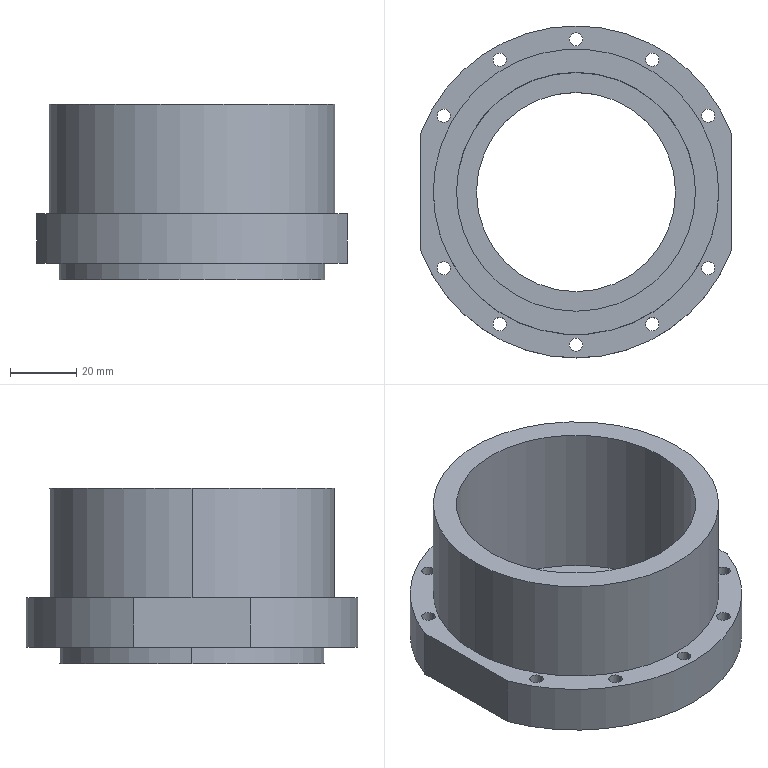Part | SolidWorks | features ICE 4, Extrusion 1 | 1 solid | 37 faces | box 93.67 x 100 x 53 mm | volume 120948 mm3 | cylinder 30 | plane 7 | commonest cylinder face diameters 4 x20 60 x2 72 x2 80 x2 86 x2 100 x2
STEP:
#1=CARTESIAN_POINT('',(-2.,46.,0.));
#2=VERTEX_POINT('',#1);
#3=CARTESIAN_POINT('',(2.,46.,0.));
#4=VERTEX_POINT('',#3);
#5=CARTESIAN_POINT('',(0.,46.,0.));
#6=DIRECTION('',(0.,0.,1.));
#7=DIRECTION('',(1.,0.,0.));
#8=AXIS2_PLACEMENT_3D('',#5,#6,#7);
#9=CIRCLE('',#8,2.);
#10=EDGE_CURVE('',#2,#4,#9,.T.);
#11=ORIENTED_EDGE('',*,*,#10,.F.);
#12=CARTESIAN_POINT('',(-2.,46.,15.));
#13=VERTEX_POINT('',#12);
#14=CARTESIAN_POINT('',(-2.,46.,-15.));
#15=DIRECTION('',(0.,0.,1.));
#16=VECTOR('',#15,1000.);
#17=LINE('',#14,#16);
#18=EDGE_CURVE('',#2,#13,#17,.T.);
#19=ORIENTED_EDGE('',*,*,#18,.T.);
#20=CARTESIAN_POINT('',(2.,46.,15.));
#21=VERTEX_POINT('',#20);
#22=CARTESIAN_POINT('',(0.,46.,15.));
#23=DIRECTION('',(0.,0.,1.));
#24=DIRECTION('',(1.,0.,0.));
#25=AXIS2_PLACEMENT_3D('',#22,#23,#24);
#26=CIRCLE('',#25,2.);
#27=EDGE_CURVE('',#13,#21,#26,.T.);
#28=ORIENTED_EDGE('',*,*,#27,.T.);
#29=CARTESIAN_POINT('',(2.,46.,-15.));
#30=DIRECTION('',(0.,0.,1.));
#31=VECTOR('',#30,1000.);
#32=LINE('',#29,#31);
#33=EDGE_CURVE('',#4,#21,#32,.T.);
#34=ORIENTED_EDGE('',*,*,#33,.F.);
#35=EDGE_LOOP('',(#11,#19,#28,#34));
#36=FACE_OUTER_BOUND('',#35,.T.);
#37=CARTESIAN_POINT('',(0.,46.,-15.));
#38=DIRECTION('',(0.,0.,1.));
#39=DIRECTION('',(1.,0.,0.));
#40=AXIS2_PLACEMENT_3D('',#37,#38,#39);
#41=CYLINDRICAL_SURFACE('',#40,2.);
#42=ADVANCED_FACE('',(#36),#41,.F.);
#43=CARTESIAN_POINT('',(-41.837,-23.,0.));
#44=VERTEX_POINT('',#43);
#45=CARTESIAN_POINT('',(-37.837,-23.,0.));
#46=VERTEX_POINT('',#45);
#47=CARTESIAN_POINT('',(-39.837,-23.,0.));
#48=DIRECTION('',(0.,0.,1.));
#49=DIRECTION('',(1.,0.,0.));
#50=AXIS2_PLACEMENT_3D('',#47,#48,#49);
#51=CIRCLE('',#50,2.);
#52=EDGE_CURVE('',#44,#46,#51,.T.);
#53=ORIENTED_EDGE('',*,*,#52,.F.);
#54=CARTESIAN_POINT('',(-41.837,-23.,15.));
#55=VERTEX_POINT('',#54);
#56=CARTESIAN_POINT('',(-41.837,-23.,-15.));
#57=DIRECTION('',(0.,0.,1.));
#58=VECTOR('',#57,1000.);
#59=LINE('',#56,#58);
#60=EDGE_CURVE('',#44,#55,#59,.T.);
#61=ORIENTED_EDGE('',*,*,#60,.T.);
#62=CARTESIAN_POINT('',(-37.837,-23.,15.));
#63=VERTEX_POINT('',#62);
#64=CARTESIAN_POINT('',(-39.837,-23.,15.));
#65=DIRECTION('',(0.,0.,1.));
#66=DIRECTION('',(-1.,0.,0.));
#67=AXIS2_PLACEMENT_3D('',#64,#65,#66);
#68=CIRCLE('',#67,2.);
#69=EDGE_CURVE('',#55,#63,#68,.T.);
#70=ORIENTED_EDGE('',*,*,#69,.T.);
#71=CARTESIAN_POINT('',(-37.837,-23.,-15.));
#72=DIRECTION('',(0.,0.,1.));
#73=VECTOR('',#72,1000.);
#74=LINE('',#71,#73);
#75=EDGE_CURVE('',#46,#63,#74,.T.);
#76=ORIENTED_EDGE('',*,*,#75,.F.);
#77=EDGE_LOOP('',(#53,#61,#70,#76));
#78=FACE_OUTER_BOUND('',#77,.T.);
#79=CARTESIAN_POINT('',(-39.837,-23.,-15.));
#80=DIRECTION('',(0.,0.,1.));
#81=DIRECTION('',(1.,0.,0.));
#82=AXIS2_PLACEMENT_3D('',#79,#80,#81);
#83=CYLINDRICAL_SURFACE('',#82,2.);
#84=ADVANCED_FACE('',(#78),#83,.F.);
#85=CARTESIAN_POINT('',(-25.,-39.837,0.));
#86=VERTEX_POINT('',#85);
#87=CARTESIAN_POINT('',(-21.,-39.837,0.));
#88=VERTEX_POINT('',#87);
#89=CARTESIAN_POINT('',(-23.,-39.837,0.));
#90=DIRECTION('',(0.,0.,1.));
#91=DIRECTION('',(1.,0.,0.));
#92=AXIS2_PLACEMENT_3D('',#89,#90,#91);
#93=CIRCLE('',#92,2.);
#94=EDGE_CURVE('',#86,#88,#93,.T.);
#95=ORIENTED_EDGE('',*,*,#94,.F.);
#96=CARTESIAN_POINT('',(-25.,-39.837,15.));
#97=VERTEX_POINT('',#96);
#98=CARTESIAN_POINT('',(-25.,-39.837,-15.));
#99=DIRECTION('',(0.,0.,1.));
#100=VECTOR('',#99,1000.);
#101=LINE('',#98,#100);
#102=EDGE_CURVE('',#86,#97,#101,.T.);
#103=ORIENTED_EDGE('',*,*,#102,.T.);
#104=CARTESIAN_POINT('',(-21.,-39.837,15.));
#105=VERTEX_POINT('',#104);
#106=CARTESIAN_POINT('',(-23.,-39.837,15.));
#107=DIRECTION('',(0.,0.,1.));
#108=DIRECTION('',(-1.,0.,0.));
#109=AXIS2_PLACEMENT_3D('',#106,#107,#108);
#110=CIRCLE('',#109,2.);
#111=EDGE_CURVE('',#97,#105,#110,.T.);
#112=ORIENTED_EDGE('',*,*,#111,.T.);
#113=CARTESIAN_POINT('',(-21.,-39.837,-15.));
#114=DIRECTION('',(0.,0.,1.));
#115=VECTOR('',#114,1000.);
#116=LINE('',#113,#115);
#117=EDGE_CURVE('',#88,#105,#116,.T.);
#118=ORIENTED_EDGE('',*,*,#117,.F.);
#119=EDGE_LOOP('',(#95,#103,#112,#118));
#120=FACE_OUTER_BOUND('',#119,.T.);
#121=CARTESIAN_POINT('',(-23.,-39.837,-15.));
#122=DIRECTION('',(0.,0.,1.));
#123=DIRECTION('',(1.,0.,0.));
#124=AXIS2_PLACEMENT_3D('',#121,#122,#123);
#125=CYLINDRICAL_SURFACE('',#124,2.);
#126=ADVANCED_FACE('',(#120),#125,.F.);
#127=CARTESIAN_POINT('',(-2.,-46.,0.));
#128=VERTEX_POINT('',#127);
#129=CARTESIAN_POINT('',(2.,-46.,0.));
#130=VERTEX_POINT('',#129);
#131=CARTESIAN_POINT('',(0.,-46.,0.));
#132=DIRECTION('',(0.,0.,1.));
#133=DIRECTION('',(1.,0.,0.));
#134=AXIS2_PLACEMENT_3D('',#131,#132,#133);
#135=CIRCLE('',#134,2.);
#136=EDGE_CURVE('',#128,#130,#135,.T.);
#137=ORIENTED_EDGE('',*,*,#136,.F.);
#138=CARTESIAN_POINT('',(-2.,-46.,15.));
#139=VERTEX_POINT('',#138);
#140=CARTESIAN_POINT('',(-2.,-46.,-15.));
#141=DIRECTION('',(0.,0.,1.));
#142=VECTOR('',#141,1000.);
#143=LINE('',#140,#142);
#144=EDGE_CURVE('',#128,#139,#143,.T.);
#145=ORIENTED_EDGE('',*,*,#144,.T.);
#146=CARTESIAN_POINT('',(2.,-46.,15.));
#147=VERTEX_POINT('',#146);
#148=CARTESIAN_POINT('',(0.,-46.,15.));
#149=DIRECTION('',(0.,0.,1.));
#150=DIRECTION('',(-1.,0.,0.));
#151=AXIS2_PLACEMENT_3D('',#148,#149,#150);
#152=CIRCLE('',#151,2.);
#153=EDGE_CURVE('',#139,#147,#152,.T.);
#154=ORIENTED_EDGE('',*,*,#153,.T.);
#155=CARTESIAN_POINT('',(2.,-46.,-15.));
#156=DIRECTION('',(0.,0.,1.));
#157=VECTOR('',#156,1000.);
#158=LINE('',#155,#157);
#159=EDGE_CURVE('',#130,#147,#158,.T.);
#160=ORIENTED_EDGE('',*,*,#159,.F.);
#161=EDGE_LOOP('',(#137,#145,#154,#160));
#162=FACE_OUTER_BOUND('',#161,.T.);
#163=CARTESIAN_POINT('',(0.,-46.,-15.));
#164=DIRECTION('',(0.,0.,1.));
#165=DIRECTION('',(1.,0.,0.));
#166=AXIS2_PLACEMENT_3D('',#163,#164,#165);
#167=CYLINDRICAL_SURFACE('',#166,2.);
#168=ADVANCED_FACE('',(#162),#167,.F.);
#169=CARTESIAN_POINT('',(21.,-39.837,0.));
#170=VERTEX_POINT('',#169);
#171=CARTESIAN_POINT('',(25.,-39.837,0.));
#172=VERTEX_POINT('',#171);
#173=CARTESIAN_POINT('',(23.,-39.837,0.));
#174=DIRECTION('',(0.,0.,1.));
#175=DIRECTION('',(1.,0.,0.));
#176=AXIS2_PLACEMENT_3D('',#173,#174,#175);
#177=CIRCLE('',#176,2.);
#178=EDGE_CURVE('',#170,#172,#177,.T.);
#179=ORIENTED_EDGE('',*,*,#178,.F.);
#180=CARTESIAN_POINT('',(21.,-39.837,15.));
#181=VERTEX_POINT('',#180);
#182=CARTESIAN_POINT('',(21.,-39.837,-15.));
#183=DIRECTION('',(0.,0.,1.));
#184=VECTOR('',#183,1000.);
#185=LINE('',#182,#184);
#186=EDGE_CURVE('',#170,#181,#185,.T.);
#187=ORIENTED_EDGE('',*,*,#186,.T.);
#188=CARTESIAN_POINT('',(25.,-39.837,15.));
#189=VERTEX_POINT('',#188);
#190=CARTESIAN_POINT('',(23.,-39.837,15.));
#191=DIRECTION('',(0.,0.,1.));
#192=DIRECTION('',(-1.,0.,0.));
#193=AXIS2_PLACEMENT_3D('',#190,#191,#192);
#194=CIRCLE('',#193,2.);
#195=EDGE_CURVE('',#181,#189,#194,.T.);
#196=ORIENTED_EDGE('',*,*,#195,.T.);
#197=CARTESIAN_POINT('',(25.,-39.837,-15.));
#198=DIRECTION('',(0.,0.,1.));
#199=VECTOR('',#198,1000.);
#200=LINE('',#197,#199);
#201=EDGE_CURVE('',#172,#189,#200,.T.);
#202=ORIENTED_EDGE('',*,*,#201,.F.);
#203=EDGE_LOOP('',(#179,#187,#196,#202));
#204=FACE_OUTER_BOUND('',#203,.T.);
#205=CARTESIAN_POINT('',(23.,-39.837,-15.));
#206=DIRECTION('',(0.,0.,1.));
#207=DIRECTION('',(1.,0.,0.));
#208=AXIS2_PLACEMENT_3D('',#205,#206,#207);
#209=CYLINDRICAL_SURFACE('',#208,2.);
#210=ADVANCED_FACE('',(#204),#209,.F.);
#211=CARTESIAN_POINT('',(37.837,-23.,0.));
#212=VERTEX_POINT('',#211);
#213=CARTESIAN_POINT('',(41.837,-23.,0.));
#214=VERTEX_POINT('',#213);
#215=CARTESIAN_POINT('',(39.837,-23.,0.));
#216=DIRECTION('',(0.,0.,1.));
#217=DIRECTION('',(1.,0.,0.));
#218=AXIS2_PLACEMENT_3D('',#215,#216,#217);
#219=CIRCLE('',#218,2.);
#220=EDGE_CURVE('',#212,#214,#219,.T.);
#221=ORIENTED_EDGE('',*,*,#220,.F.);
#222=CARTESIAN_POINT('',(37.837,-23.,15.));
#223=VERTEX_POINT('',#222);
#224=CARTESIAN_POINT('',(37.837,-23.,-15.));
#225=DIRECTION('',(0.,0.,1.));
#226=VECTOR('',#225,1000.);
#227=LINE('',#224,#226);
#228=EDGE_CURVE('',#212,#223,#227,.T.);
#229=ORIENTED_EDGE('',*,*,#228,.T.);
#230=CARTESIAN_POINT('',(41.837,-23.,15.));
#231=VERTEX_POINT('',#230);
#232=CARTESIAN_POINT('',(39.837,-23.,15.));
#233=DIRECTION('',(0.,0.,1.));
#234=DIRECTION('',(-1.,0.,0.));
#235=AXIS2_PLACEMENT_3D('',#232,#233,#234);
#236=CIRCLE('',#235,2.);
#237=EDGE_CURVE('',#223,#231,#236,.T.);
#238=ORIENTED_EDGE('',*,*,#237,.T.);
#239=CARTESIAN_POINT('',(41.837,-23.,-15.));
#240=DIRECTION('',(0.,0.,1.));
#241=VECTOR('',#240,1000.);
#242=LINE('',#239,#241);
#243=EDGE_CURVE('',#214,#231,#242,.T.);
#244=ORIENTED_EDGE('',*,*,#243,.F.);
#245=EDGE_LOOP('',(#221,#229,#238,#244));
#246=FACE_OUTER_BOUND('',#245,.T.);
#247=CARTESIAN_POINT('',(39.837,-23.,-15.));
#248=DIRECTION('',(0.,0.,1.));
#249=DIRECTION('',(1.,0.,0.));
#250=AXIS2_PLACEMENT_3D('',#247,#248,#249);
#251=CYLINDRICAL_SURFACE('',#250,2.);
#252=ADVANCED_FACE('',(#246),#251,.F.);
#253=CARTESIAN_POINT('',(-41.837,23.,0.));
#254=VERTEX_POINT('',#253);
#255=CARTESIAN_POINT('',(-37.837,23.,0.));
#256=VERTEX_POINT('',#255);
#257=CARTESIAN_POINT('',(-39.837,23.,0.));
#258=DIRECTION('',(0.,0.,1.));
#259=DIRECTION('',(1.,0.,0.));
#260=AXIS2_PLACEMENT_3D('',#257,#258,#259);
#261=CIRCLE('',#260,2.);
#262=EDGE_CURVE('',#254,#256,#261,.T.);
#263=ORIENTED_EDGE('',*,*,#262,.F.);
#264=CARTESIAN_POINT('',(-41.837,23.,15.));
#265=VERTEX_POINT('',#264);
#266=CARTESIAN_POINT('',(-41.837,23.,-15.));
#267=DIRECTION('',(0.,0.,1.));
#268=VECTOR('',#267,1000.);
#269=LINE('',#266,#268);
#270=EDGE_CURVE('',#254,#265,#269,.T.);
#271=ORIENTED_EDGE('',*,*,#270,.T.);
#272=CARTESIAN_POINT('',(-37.837,23.,15.));
#273=VERTEX_POINT('',#272);
#274=CARTESIAN_POINT('',(-39.837,23.,15.));
#275=DIRECTION('',(0.,0.,1.));
#276=DIRECTION('',(1.,0.,0.));
#277=AXIS2_PLACEMENT_3D('',#274,#275,#276);
#278=CIRCLE('',#277,2.);
#279=EDGE_CURVE('',#265,#273,#278,.T.);
#280=ORIENTED_EDGE('',*,*,#279,.T.);
#281=CARTESIAN_POINT('',(-37.837,23.,-15.));
#282=DIRECTION('',(0.,0.,1.));
#283=VECTOR('',#282,1000.);
#284=LINE('',#281,#283);
#285=EDGE_CURVE('',#256,#273,#284,.T.);
#286=ORIENTED_EDGE('',*,*,#285,.F.);
#287=EDGE_LOOP('',(#263,#271,#280,#286));
#288=FACE_OUTER_BOUND('',#287,.T.);
#289=CARTESIAN_POINT('',(-39.837,23.,-15.));
#290=DIRECTION('',(0.,0.,1.));
#291=DIRECTION('',(1.,0.,0.));
#292=AXIS2_PLACEMENT_3D('',#289,#290,#291);
#293=CYLINDRICAL_SURFACE('',#292,2.);
#294=ADVANCED_FACE('',(#288),#293,.F.);
#295=CARTESIAN_POINT('',(-25.,39.837,0.));
#296=VERTEX_POINT('',#295);
#297=CARTESIAN_POINT('',(-21.,39.837,0.));
#298=VERTEX_POINT('',#297);
#299=CARTESIAN_POINT('',(-23.,39.837,0.));
#300=DIRECTION('',(0.,0.,1.));
#301=DIRECTION('',(1.,0.,0.));
#302=AXIS2_PLACEMENT_3D('',#299,#300,#301);
#303=CIRCLE('',#302,2.);
#304=EDGE_CURVE('',#296,#298,#303,.T.);
#305=ORIENTED_EDGE('',*,*,#304,.F.);
#306=CARTESIAN_POINT('',(-25.,39.837,15.));
#307=VERTEX_POINT('',#306);
#308=CARTESIAN_POINT('',(-25.,39.837,-15.));
#309=DIRECTION('',(0.,0.,1.));
#310=VECTOR('',#309,1000.);
#311=LINE('',#308,#310);
#312=EDGE_CURVE('',#296,#307,#311,.T.);
#313=ORIENTED_EDGE('',*,*,#312,.T.);
#314=CARTESIAN_POINT('',(-21.,39.837,15.));
#315=VERTEX_POINT('',#314);
#316=CARTESIAN_POINT('',(-23.,39.837,15.));
#317=DIRECTION('',(0.,0.,1.));
#318=DIRECTION('',(1.,0.,0.));
#319=AXIS2_PLACEMENT_3D('',#316,#317,#318);
#320=CIRCLE('',#319,2.);
#321=EDGE_CURVE('',#307,#315,#320,.T.);
#322=ORIENTED_EDGE('',*,*,#321,.T.);
#323=CARTESIAN_POINT('',(-21.,39.837,-15.));
#324=DIRECTION('',(0.,0.,1.));
#325=VECTOR('',#324,1000.);
#326=LINE('',#323,#325);
#327=EDGE_CURVE('',#298,#315,#326,.T.);
#328=ORIENTED_EDGE('',*,*,#327,.F.);
#329=EDGE_LOOP('',(#305,#313,#322,#328));
#330=FACE_OUTER_BOUND('',#329,.T.);
#331=CARTESIAN_POINT('',(-23.,39.837,-15.));
#332=DIRECTION('',(0.,0.,1.));
#333=DIRECTION('',(1.,0.,0.));
#334=AXIS2_PLACEMENT_3D('',#331,#332,#333);
#335=CYLINDRICAL_SURFACE('',#334,2.);
#336=ADVANCED_FACE('',(#330),#335,.F.);
#337=CARTESIAN_POINT('',(37.837,23.,0.));
#338=VERTEX_POINT('',#337);
#339=CARTESIAN_POINT('',(41.837,23.,0.));
#340=VERTEX_POINT('',#339);
#341=CARTESIAN_POINT('',(39.837,23.,0.));
#342=DIRECTION('',(0.,0.,1.));
#343=DIRECTION('',(1.,0.,0.));
#344=AXIS2_PLACEMENT_3D('',#341,#342,#343);
#345=CIRCLE('',#344,2.);
#346=EDGE_CURVE('',#338,#340,#345,.T.);
#347=ORIENTED_EDGE('',*,*,#346,.F.);
#348=CARTESIAN_POINT('',(37.837,23.,15.));
#349=VERTEX_POINT('',#348);
#350=CARTESIAN_POINT('',(37.837,23.,-15.));
#351=DIRECTION('',(0.,0.,1.));
#352=VECTOR('',#351,1000.);
#353=LINE('',#350,#352);
#354=EDGE_CURVE('',#338,#349,#353,.T.);
#355=ORIENTED_EDGE('',*,*,#354,.T.);
#356=CARTESIAN_POINT('',(41.837,23.,15.));
#357=VERTEX_POINT('',#356);
#358=CARTESIAN_POINT('',(39.837,23.,15.));
#359=DIRECTION('',(0.,0.,1.));
#360=DIRECTION('',(1.,0.,0.));
#361=AXIS2_PLACEMENT_3D('',#358,#359,#360);
#362=CIRCLE('',#361,2.);
#363=EDGE_CURVE('',#349,#357,#362,.T.);
#364=ORIENTED_EDGE('',*,*,#363,.T.);
#365=CARTESIAN_POINT('',(41.837,23.,-15.));
#366=DIRECTION('',(0.,0.,1.));
#367=VECTOR('',#366,1000.);
#368=LINE('',#365,#367);
#369=EDGE_CURVE('',#340,#357,#368,.T.);
#370=ORIENTED_EDGE('',*,*,#369,.F.);
#371=EDGE_LOOP('',(#347,#355,#364,#370));
#372=FACE_OUTER_BOUND('',#371,.T.);
#373=CARTESIAN_POINT('',(39.837,23.,-15.));
#374=DIRECTION('',(0.,0.,1.));
#375=DIRECTION('',(1.,0.,0.));
#376=AXIS2_PLACEMENT_3D('',#373,#374,#375);
#377=CYLINDRICAL_SURFACE('',#376,2.);
#378=ADVANCED_FACE('',(#372),#377,.F.);
#379=CARTESIAN_POINT('',(21.,39.837,0.));
#380=VERTEX_POINT('',#379);
#381=CARTESIAN_POINT('',(25.,39.837,0.));
#382=VERTEX_POINT('',#381);
#383=CARTESIAN_POINT('',(23.,39.837,0.));
#384=DIRECTION('',(0.,0.,1.));
#385=DIRECTION('',(1.,0.,0.));
#386=AXIS2_PLACEMENT_3D('',#383,#384,#385);
#387=CIRCLE('',#386,2.);
#388=EDGE_CURVE('',#380,#382,#387,.T.);
#389=ORIENTED_EDGE('',*,*,#388,.F.);
#390=CARTESIAN_POINT('',(21.,39.837,15.));
#391=VERTEX_POINT('',#390);
#392=CARTESIAN_POINT('',(21.,39.837,-15.));
#393=DIRECTION('',(0.,0.,1.));
#394=VECTOR('',#393,1000.);
#395=LINE('',#392,#394);
#396=EDGE_CURVE('',#380,#391,#395,.T.);
#397=ORIENTED_EDGE('',*,*,#396,.T.);
#398=CARTESIAN_POINT('',(25.,39.837,15.));
#399=VERTEX_POINT('',#398);
#400=CARTESIAN_POINT('',(23.,39.837,15.));
#401=DIRECTION('',(0.,0.,1.));
#402=DIRECTION('',(1.,0.,0.));
#403=AXIS2_PLACEMENT_3D('',#400,#401,#402);
#404=CIRCLE('',#403,2.);
#405=EDGE_CURVE('',#391,#399,#404,.T.);
#406=ORIENTED_EDGE('',*,*,#405,.T.);
#407=CARTESIAN_POINT('',(25.,39.837,-15.));
#408=DIRECTION('',(0.,0.,1.));
#409=VECTOR('',#408,1000.);
#410=LINE('',#407,#409);
#411=EDGE_CURVE('',#382,#399,#410,.T.);
#412=ORIENTED_EDGE('',*,*,#411,.F.);
#413=EDGE_LOOP('',(#389,#397,#406,#412));
#414=FACE_OUTER_BOUND('',#413,.T.);
#415=CARTESIAN_POINT('',(23.,39.837,-15.));
#416=DIRECTION('',(0.,0.,1.));
#417=DIRECTION('',(1.,0.,0.));
#418=AXIS2_PLACEMENT_3D('',#415,#416,#417);
#419=CYLINDRICAL_SURFACE('',#418,2.);
#420=ADVANCED_FACE('',(#414),#419,.F.);
#421=CARTESIAN_POINT('',(43.,0.,48.));
#422=VERTEX_POINT('',#421);
#423=CARTESIAN_POINT('',(-43.,0.,48.));
#424=VERTEX_POINT('',#423);
#425=CARTESIAN_POINT('',(0.,0.,48.));
#426=DIRECTION('',(0.,0.,1.));
#427=DIRECTION('',(1.,0.,0.));
#428=AXIS2_PLACEMENT_3D('',#425,#426,#427);
#429=CIRCLE('',#428,43.);
#430=EDGE_CURVE('',#422,#424,#429,.T.);
#431=ORIENTED_EDGE('',*,*,#430,.F.);
#432=CARTESIAN_POINT('',(43.,0.,15.));
#433=VERTEX_POINT('',#432);
#434=CARTESIAN_POINT('',(43.,0.,48.));
#435=DIRECTION('',(0.,0.,-1.));
#436=VECTOR('',#435,1000.);
#437=LINE('',#434,#436);
#438=EDGE_CURVE('',#422,#433,#437,.T.);
#439=ORIENTED_EDGE('',*,*,#438,.T.);
#440=CARTESIAN_POINT('',(-43.,0.,15.));
#441=VERTEX_POINT('',#440);
#442=CARTESIAN_POINT('',(0.,0.,15.));
#443=DIRECTION('',(0.,0.,1.));
#444=DIRECTION('',(1.,0.,0.));
#445=AXIS2_PLACEMENT_3D('',#442,#443,#444);
#446=CIRCLE('',#445,43.);
#447=EDGE_CURVE('',#433,#441,#446,.T.);
#448=ORIENTED_EDGE('',*,*,#447,.T.);
#449=CARTESIAN_POINT('',(-43.,0.,48.));
#450=DIRECTION('',(0.,0.,-1.));
#451=VECTOR('',#450,1000.);
#452=LINE('',#449,#451);
#453=EDGE_CURVE('',#424,#441,#452,.T.);
#454=ORIENTED_EDGE('',*,*,#453,.F.);
#455=EDGE_LOOP('',(#431,#439,#448,#454));
#456=FACE_OUTER_BOUND('',#455,.T.);
#457=CARTESIAN_POINT('',(0.,0.,48.));
#458=DIRECTION('',(0.,0.,-1.));
#459=DIRECTION('',(-1.,0.,0.));
#460=AXIS2_PLACEMENT_3D('',#457,#458,#459);
#461=CYLINDRICAL_SURFACE('',#460,43.);
#462=ADVANCED_FACE('',(#456),#461,.T.);
#463=CARTESIAN_POINT('',(30.,0.,-5.));
#464=VERTEX_POINT('',#463);
#465=CARTESIAN_POINT('',(-30.,0.,-5.));
#466=VERTEX_POINT('',#465);
#467=CARTESIAN_POINT('',(0.,0.,-5.));
#468=DIRECTION('',(0.,0.,-1.));
#469=DIRECTION('',(-1.,0.,0.));
#470=AXIS2_PLACEMENT_3D('',#467,#468,#469);
#471=CIRCLE('',#470,30.);
#472=EDGE_CURVE('',#464,#466,#471,.T.);
#473=ORIENTED_EDGE('',*,*,#472,.T.);
#474=CARTESIAN_POINT('',(-30.,0.,0.));
#475=VERTEX_POINT('',#474);
#476=CARTESIAN_POINT('',(-30.,0.,-5.));
#477=DIRECTION('',(0.,0.,1.));
#478=VECTOR('',#477,1000.);
#479=LINE('',#476,#478);
#480=EDGE_CURVE('',#466,#475,#479,.T.);
#481=ORIENTED_EDGE('',*,*,#480,.T.);
#482=CARTESIAN_POINT('',(30.,0.,0.));
#483=VERTEX_POINT('',#482);
#484=CARTESIAN_POINT('',(0.,0.,0.));
#485=DIRECTION('',(0.,0.,-1.));
#486=DIRECTION('',(-1.,0.,0.));
#487=AXIS2_PLACEMENT_3D('',#484,#485,#486);
#488=CIRCLE('',#487,30.);
#489=EDGE_CURVE('',#483,#475,#488,.T.);
#490=ORIENTED_EDGE('',*,*,#489,.F.);
#491=CARTESIAN_POINT('',(30.,0.,-5.));
#492=DIRECTION('',(0.,0.,1.));
#493=VECTOR('',#492,1000.);
#494=LINE('',#491,#493);
#495=EDGE_CURVE('',#464,#483,#494,.T.);
#496=ORIENTED_EDGE('',*,*,#495,.F.);
#497=EDGE_LOOP('',(#473,#481,#490,#496));
#498=FACE_OUTER_BOUND('',#497,.T.);
#499=CARTESIAN_POINT('',(0.,0.,-5.));
#500=DIRECTION('',(0.,0.,1.));
#501=DIRECTION('',(1.,0.,0.));
#502=AXIS2_PLACEMENT_3D('',#499,#500,#501);
#503=CYLINDRICAL_SURFACE('',#502,30.);
#504=ADVANCED_FACE('',(#498),#503,.F.);
#505=CARTESIAN_POINT('',(-40.,0.,-5.));
#506=VERTEX_POINT('',#505);
#507=CARTESIAN_POINT('',(40.,0.,-5.));
#508=VERTEX_POINT('',#507);
#509=CARTESIAN_POINT('',(0.,0.,-5.));
#510=DIRECTION('',(0.,0.,-1.));
#511=DIRECTION('',(-1.,0.,0.));
#512=AXIS2_PLACEMENT_3D('',#509,#510,#511);
#513=CIRCLE('',#512,40.);
#514=EDGE_CURVE('',#506,#508,#513,.T.);
#515=ORIENTED_EDGE('',*,*,#514,.F.);
#516=CARTESIAN_POINT('',(-40.,0.,0.));
#517=VERTEX_POINT('',#516);
#518=CARTESIAN_POINT('',(-40.,0.,-5.));
#519=DIRECTION('',(0.,0.,1.));
#520=VECTOR('',#519,1000.);
#521=LINE('',#518,#520);
#522=EDGE_CURVE('',#506,#517,#521,.T.);
#523=ORIENTED_EDGE('',*,*,#522,.T.);
#524=CARTESIAN_POINT('',(40.,0.,0.));
#525=VERTEX_POINT('',#524);
#526=CARTESIAN_POINT('',(0.,0.,0.));
#527=DIRECTION('',(0.,0.,-1.));
#528=DIRECTION('',(1.,0.,0.));
#529=AXIS2_PLACEMENT_3D('',#526,#527,#528);
#530=CIRCLE('',#529,40.);
#531=EDGE_CURVE('',#517,#525,#530,.T.);
#532=ORIENTED_EDGE('',*,*,#531,.T.);
#533=CARTESIAN_POINT('',(40.,0.,-5.));
#534=DIRECTION('',(0.,0.,1.));
#535=VECTOR('',#534,1000.);
#536=LINE('',#533,#535);
#537=EDGE_CURVE('',#508,#525,#536,.T.);
#538=ORIENTED_EDGE('',*,*,#537,.F.);
#539=EDGE_LOOP('',(#515,#523,#532,#538));
#540=FACE_OUTER_BOUND('',#539,.T.);
#541=CARTESIAN_POINT('',(0.,0.,-5.));
#542=DIRECTION('',(0.,0.,1.));
#543=DIRECTION('',(1.,0.,0.));
#544=AXIS2_PLACEMENT_3D('',#541,#542,#543);
#545=CYLINDRICAL_SURFACE('',#544,40.);
#546=ADVANCED_FACE('',(#540),#545,.T.);
#547=CARTESIAN_POINT('',(-36.,0.,48.));
#548=VERTEX_POINT('',#547);
#549=CARTESIAN_POINT('',(36.,0.,48.));
#550=VERTEX_POINT('',#549);
#551=CARTESIAN_POINT('',(0.,0.,48.));
#552=DIRECTION('',(0.,0.,1.));
#553=DIRECTION('',(1.,0.,0.));
#554=AXIS2_PLACEMENT_3D('',#551,#552,#553);
#555=CIRCLE('',#554,36.);
#556=EDGE_CURVE('',#548,#550,#555,.T.);
#557=ORIENTED_EDGE('',*,*,#556,.T.);
#558=CARTESIAN_POINT('',(36.,0.,0.));
#559=VERTEX_POINT('',#558);
#560=CARTESIAN_POINT('',(36.,0.,15.));
#561=DIRECTION('',(0.,0.,-1.));
#562=VECTOR('',#561,1000.);
#563=LINE('',#560,#562);
#564=EDGE_CURVE('',#550,#559,#563,.T.);
#565=ORIENTED_EDGE('',*,*,#564,.T.);
#566=CARTESIAN_POINT('',(-36.,0.,0.));
#567=VERTEX_POINT('',#566);
#568=CARTESIAN_POINT('',(0.,0.,0.));
#569=DIRECTION('',(0.,0.,1.));
#570=DIRECTION('',(1.,0.,0.));
#571=AXIS2_PLACEMENT_3D('',#568,#569,#570);
#572=CIRCLE('',#571,36.);
#573=EDGE_CURVE('',#567,#559,#572,.T.);
#574=ORIENTED_EDGE('',*,*,#573,.F.);
#575=CARTESIAN_POINT('',(-36.,0.,15.));
#576=DIRECTION('',(0.,0.,-1.));
#577=VECTOR('',#576,1000.);
#578=LINE('',#575,#577);
#579=EDGE_CURVE('',#548,#567,#578,.T.);
#580=ORIENTED_EDGE('',*,*,#579,.F.);
#581=EDGE_LOOP('',(#557,#565,#574,#580));
#582=FACE_OUTER_BOUND('',#581,.T.);
#583=CARTESIAN_POINT('',(0.,0.,15.));
#584=DIRECTION('',(0.,0.,-1.));
#585=DIRECTION('',(-1.,0.,0.));
#586=AXIS2_PLACEMENT_3D('',#583,#584,#585);
#587=CYLINDRICAL_SURFACE('',#586,36.);
#588=ADVANCED_FACE('',(#582),#587,.F.);
#589=CARTESIAN_POINT('',(-46.835,-17.507,15.));
#590=VERTEX_POINT('',#589);
#591=CARTESIAN_POINT('',(46.835,-17.507,15.));
#592=VERTEX_POINT('',#591);
#593=CARTESIAN_POINT('',(0.,0.,15.));
#594=DIRECTION('',(0.,0.,1.));
#595=DIRECTION('',(1.,0.,0.));
#596=AXIS2_PLACEMENT_3D('',#593,#594,#595);
#597=CIRCLE('',#596,50.);
#598=EDGE_CURVE('',#590,#592,#597,.T.);
#599=ORIENTED_EDGE('',*,*,#598,.F.);
#600=CARTESIAN_POINT('',(-46.835,-17.507,0.));
#601=VERTEX_POINT('',#600);
#602=CARTESIAN_POINT('',(-46.835,-17.507,15.));
#603=DIRECTION('',(0.,0.,-1.));
#604=VECTOR('',#603,1000.);
#605=LINE('',#602,#604);
#606=EDGE_CURVE('',#590,#601,#605,.T.);
#607=ORIENTED_EDGE('',*,*,#606,.T.);
#608=CARTESIAN_POINT('',(46.835,-17.507,0.));
#609=VERTEX_POINT('',#608);
#610=CARTESIAN_POINT('',(0.,0.,0.));
#611=DIRECTION('',(0.,0.,1.));
#612=DIRECTION('',(1.,0.,0.));
#613=AXIS2_PLACEMENT_3D('',#610,#611,#612);
#614=CIRCLE('',#613,50.);
#615=EDGE_CURVE('',#601,#609,#614,.T.);
#616=ORIENTED_EDGE('',*,*,#615,.T.);
#617=CARTESIAN_POINT('',(46.835,-17.507,15.));
#618=DIRECTION('',(0.,0.,1.));
#619=VECTOR('',#618,1000.);
#620=LINE('',#617,#619);
#621=EDGE_CURVE('',#609,#592,#620,.T.);
#622=ORIENTED_EDGE('',*,*,#621,.T.);
#623=EDGE_LOOP('',(#599,#607,#616,#622));
#624=FACE_OUTER_BOUND('',#623,.T.);
#625=CARTESIAN_POINT('',(0.,0.,15.));
#626=DIRECTION('',(0.,0.,-1.));
#627=DIRECTION('',(-1.,0.,0.));
#628=AXIS2_PLACEMENT_3D('',#625,#626,#627);
#629=CYLINDRICAL_SURFACE('',#628,50.);
#630=ADVANCED_FACE('',(#624),#629,.T.);
#631=CARTESIAN_POINT('',(0.,46.,15.));
#632=DIRECTION('',(0.,0.,1.));
#633=DIRECTION('',(1.,0.,0.));
#634=AXIS2_PLACEMENT_3D('',#631,#632,#633);
#635=CIRCLE('',#634,2.);
#636=EDGE_CURVE('',#21,#13,#635,.T.);
#637=ORIENTED_EDGE('',*,*,#636,.F.);
#638=ORIENTED_EDGE('',*,*,#27,.F.);
#639=EDGE_LOOP('',(#637,#638));
#640=FACE_BOUND('',#639,.T.);
#641=CARTESIAN_POINT('',(-39.837,-23.,15.));
#642=DIRECTION('',(0.,0.,1.));
#643=DIRECTION('',(-1.,0.,0.));
#644=AXIS2_PLACEMENT_3D('',#641,#642,#643);
#645=CIRCLE('',#644,2.);
#646=EDGE_CURVE('',#63,#55,#645,.T.);
#647=ORIENTED_EDGE('',*,*,#646,.F.);
#648=ORIENTED_EDGE('',*,*,#69,.F.);
#649=EDGE_LOOP('',(#647,#648));
#650=FACE_BOUND('',#649,.T.);
#651=CARTESIAN_POINT('',(-23.,-39.837,15.));
#652=DIRECTION('',(0.,0.,1.));
#653=DIRECTION('',(-1.,0.,0.));
#654=AXIS2_PLACEMENT_3D('',#651,#652,#653);
#655=CIRCLE('',#654,2.);
#656=EDGE_CURVE('',#105,#97,#655,.T.);
#657=ORIENTED_EDGE('',*,*,#656,.F.);
#658=ORIENTED_EDGE('',*,*,#111,.F.);
#659=EDGE_LOOP('',(#657,#658));
#660=FACE_BOUND('',#659,.T.);
#661=CARTESIAN_POINT('',(0.,-46.,15.));
#662=DIRECTION('',(0.,0.,1.));
#663=DIRECTION('',(-1.,0.,0.));
#664=AXIS2_PLACEMENT_3D('',#661,#662,#663);
#665=CIRCLE('',#664,2.);
#666=EDGE_CURVE('',#147,#139,#665,.T.);
#667=ORIENTED_EDGE('',*,*,#666,.F.);
#668=ORIENTED_EDGE('',*,*,#153,.F.);
#669=EDGE_LOOP('',(#667,#668));
#670=FACE_BOUND('',#669,.T.);
#671=CARTESIAN_POINT('',(23.,-39.837,15.));
#672=DIRECTION('',(0.,0.,1.));
#673=DIRECTION('',(-1.,0.,0.));
#674=AXIS2_PLACEMENT_3D('',#671,#672,#673);
#675=CIRCLE('',#674,2.);
#676=EDGE_CURVE('',#189,#181,#675,.T.);
#677=ORIENTED_EDGE('',*,*,#676,.F.);
#678=ORIENTED_EDGE('',*,*,#195,.F.);
#679=EDGE_LOOP('',(#677,#678));
#680=FACE_BOUND('',#679,.T.);
#681=CARTESIAN_POINT('',(39.837,-23.,15.));
#682=DIRECTION('',(0.,0.,1.));
#683=DIRECTION('',(-1.,0.,0.));
#684=AXIS2_PLACEMENT_3D('',#681,#682,#683);
#685=CIRCLE('',#684,2.);
#686=EDGE_CURVE('',#231,#223,#685,.T.);
#687=ORIENTED_EDGE('',*,*,#686,.F.);
#688=ORIENTED_EDGE('',*,*,#237,.F.);
#689=EDGE_LOOP('',(#687,#688));
#690=FACE_BOUND('',#689,.T.);
#691=CARTESIAN_POINT('',(-39.837,23.,15.));
#692=DIRECTION('',(0.,0.,1.));
#693=DIRECTION('',(1.,0.,0.));
#694=AXIS2_PLACEMENT_3D('',#691,#692,#693);
#695=CIRCLE('',#694,2.);
#696=EDGE_CURVE('',#273,#265,#695,.T.);
#697=ORIENTED_EDGE('',*,*,#696,.F.);
#698=ORIENTED_EDGE('',*,*,#279,.F.);
#699=EDGE_LOOP('',(#697,#698));
#700=FACE_BOUND('',#699,.T.);
#701=CARTESIAN_POINT('',(-23.,39.837,15.));
#702=DIRECTION('',(0.,0.,1.));
#703=DIRECTION('',(1.,0.,0.));
#704=AXIS2_PLACEMENT_3D('',#701,#702,#703);
#705=CIRCLE('',#704,2.);
#706=EDGE_CURVE('',#315,#307,#705,.T.);
#707=ORIENTED_EDGE('',*,*,#706,.F.);
#708=ORIENTED_EDGE('',*,*,#321,.F.);
#709=EDGE_LOOP('',(#707,#708));
#710=FACE_BOUND('',#709,.T.);
#711=CARTESIAN_POINT('',(39.837,23.,15.));
#712=DIRECTION('',(0.,0.,1.));
#713=DIRECTION('',(1.,0.,0.));
#714=AXIS2_PLACEMENT_3D('',#711,#712,#713);
#715=CIRCLE('',#714,2.);
#716=EDGE_CURVE('',#357,#349,#715,.T.);
#717=ORIENTED_EDGE('',*,*,#716,.F.);
#718=ORIENTED_EDGE('',*,*,#363,.F.);
#719=EDGE_LOOP('',(#717,#718));
#720=FACE_BOUND('',#719,.T.);
#721=CARTESIAN_POINT('',(23.,39.837,15.));
#722=DIRECTION('',(0.,0.,1.));
#723=DIRECTION('',(1.,0.,0.));
#724=AXIS2_PLACEMENT_3D('',#721,#722,#723);
#725=CIRCLE('',#724,2.);
#726=EDGE_CURVE('',#399,#391,#725,.T.);
#727=ORIENTED_EDGE('',*,*,#726,.F.);
#728=ORIENTED_EDGE('',*,*,#405,.F.);
#729=EDGE_LOOP('',(#727,#728));
#730=FACE_BOUND('',#729,.T.);
#731=CARTESIAN_POINT('',(0.,0.,15.));
#732=DIRECTION('',(0.,0.,1.));
#733=DIRECTION('',(1.,0.,0.));
#734=AXIS2_PLACEMENT_3D('',#731,#732,#733);
#735=CIRCLE('',#734,43.);
#736=EDGE_CURVE('',#441,#433,#735,.T.);
#737=ORIENTED_EDGE('',*,*,#736,.F.);
#738=ORIENTED_EDGE('',*,*,#447,.F.);
#739=EDGE_LOOP('',(#737,#738));
#740=FACE_BOUND('',#739,.T.);
#741=CARTESIAN_POINT('',(-46.835,17.507,15.));
#742=VERTEX_POINT('',#741);
#743=CARTESIAN_POINT('',(-46.835,17.507,15.));
#744=DIRECTION('',(0.,1.,0.));
#745=VECTOR('',#744,1000.);
#746=LINE('',#743,#745);
#747=EDGE_CURVE('',#590,#742,#746,.T.);
#748=ORIENTED_EDGE('',*,*,#747,.F.);
#749=ORIENTED_EDGE('',*,*,#598,.T.);
#750=CARTESIAN_POINT('',(46.835,17.507,15.));
#751=VERTEX_POINT('',#750);
#752=CARTESIAN_POINT('',(46.835,17.507,15.));
#753=DIRECTION('',(0.,-1.,0.));
#754=VECTOR('',#753,1000.);
#755=LINE('',#752,#754);
#756=EDGE_CURVE('',#751,#592,#755,.T.);
#757=ORIENTED_EDGE('',*,*,#756,.F.);
#758=CARTESIAN_POINT('',(0.,0.,15.));
#759=DIRECTION('',(0.,0.,1.));
#760=DIRECTION('',(1.,0.,0.));
#761=AXIS2_PLACEMENT_3D('',#758,#759,#760);
#762=CIRCLE('',#761,50.);
#763=EDGE_CURVE('',#751,#742,#762,.T.);
#764=ORIENTED_EDGE('',*,*,#763,.T.);
#765=EDGE_LOOP('',(#748,#749,#757,#764));
#766=FACE_OUTER_BOUND('',#765,.T.);
#767=CARTESIAN_POINT('',(0.,0.,15.));
#768=DIRECTION('',(0.,0.,1.));
#769=DIRECTION('',(1.,0.,0.));
#770=AXIS2_PLACEMENT_3D('',#767,#768,#769);
#771=PLANE('',#770);
#772=ADVANCED_FACE('',(#640,#650,#660,#670,#680,#690,#700,#710,#720,#730,#740,#766),#771,.T.);
#773=CARTESIAN_POINT('',(0.,46.,0.));
#774=DIRECTION('',(0.,0.,1.));
#775=DIRECTION('',(1.,0.,0.));
#776=AXIS2_PLACEMENT_3D('',#773,#774,#775);
#777=CIRCLE('',#776,2.);
#778=EDGE_CURVE('',#4,#2,#777,.T.);
#779=ORIENTED_EDGE('',*,*,#778,.T.);
#780=ORIENTED_EDGE('',*,*,#10,.T.);
#781=EDGE_LOOP('',(#779,#780));
#782=FACE_BOUND('',#781,.T.);
#783=CARTESIAN_POINT('',(-39.837,-23.,0.));
#784=DIRECTION('',(0.,0.,1.));
#785=DIRECTION('',(1.,0.,0.));
#786=AXIS2_PLACEMENT_3D('',#783,#784,#785);
#787=CIRCLE('',#786,2.);
#788=EDGE_CURVE('',#46,#44,#787,.T.);
#789=ORIENTED_EDGE('',*,*,#788,.T.);
#790=ORIENTED_EDGE('',*,*,#52,.T.);
#791=EDGE_LOOP('',(#789,#790));
#792=FACE_BOUND('',#791,.T.);
#793=CARTESIAN_POINT('',(-23.,-39.837,0.));
#794=DIRECTION('',(0.,0.,1.));
#795=DIRECTION('',(1.,0.,0.));
#796=AXIS2_PLACEMENT_3D('',#793,#794,#795);
#797=CIRCLE('',#796,2.);
#798=EDGE_CURVE('',#88,#86,#797,.T.);
#799=ORIENTED_EDGE('',*,*,#798,.T.);
#800=ORIENTED_EDGE('',*,*,#94,.T.);
#801=EDGE_LOOP('',(#799,#800));
#802=FACE_BOUND('',#801,.T.);
#803=CARTESIAN_POINT('',(0.,-46.,0.));
#804=DIRECTION('',(0.,0.,1.));
#805=DIRECTION('',(1.,0.,0.));
#806=AXIS2_PLACEMENT_3D('',#803,#804,#805);
#807=CIRCLE('',#806,2.);
#808=EDGE_CURVE('',#130,#128,#807,.T.);
#809=ORIENTED_EDGE('',*,*,#808,.T.);
#810=ORIENTED_EDGE('',*,*,#136,.T.);
#811=EDGE_LOOP('',(#809,#810));
#812=FACE_BOUND('',#811,.T.);
#813=CARTESIAN_POINT('',(23.,-39.837,0.));
#814=DIRECTION('',(0.,0.,1.));
#815=DIRECTION('',(1.,0.,0.));
#816=AXIS2_PLACEMENT_3D('',#813,#814,#815);
#817=CIRCLE('',#816,2.);
#818=EDGE_CURVE('',#172,#170,#817,.T.);
#819=ORIENTED_EDGE('',*,*,#818,.T.);
#820=ORIENTED_EDGE('',*,*,#178,.T.);
#821=EDGE_LOOP('',(#819,#820));
#822=FACE_BOUND('',#821,.T.);
#823=CARTESIAN_POINT('',(39.837,-23.,0.));
#824=DIRECTION('',(0.,0.,1.));
#825=DIRECTION('',(1.,0.,0.));
#826=AXIS2_PLACEMENT_3D('',#823,#824,#825);
#827=CIRCLE('',#826,2.);
#828=EDGE_CURVE('',#214,#212,#827,.T.);
#829=ORIENTED_EDGE('',*,*,#828,.T.);
#830=ORIENTED_EDGE('',*,*,#220,.T.);
#831=EDGE_LOOP('',(#829,#830));
#832=FACE_BOUND('',#831,.T.);
#833=CARTESIAN_POINT('',(-39.837,23.,0.));
#834=DIRECTION('',(0.,0.,1.));
#835=DIRECTION('',(1.,0.,0.));
#836=AXIS2_PLACEMENT_3D('',#833,#834,#835);
#837=CIRCLE('',#836,2.);
#838=EDGE_CURVE('',#256,#254,#837,.T.);
#839=ORIENTED_EDGE('',*,*,#838,.T.);
#840=ORIENTED_EDGE('',*,*,#262,.T.);
#841=EDGE_LOOP('',(#839,#840));
#842=FACE_BOUND('',#841,.T.);
#843=CARTESIAN_POINT('',(-23.,39.837,0.));
#844=DIRECTION('',(0.,0.,1.));
#845=DIRECTION('',(1.,0.,0.));
#846=AXIS2_PLACEMENT_3D('',#843,#844,#845);
#847=CIRCLE('',#846,2.);
#848=EDGE_CURVE('',#298,#296,#847,.T.);
#849=ORIENTED_EDGE('',*,*,#848,.T.);
#850=ORIENTED_EDGE('',*,*,#304,.T.);
#851=EDGE_LOOP('',(#849,#850));
#852=FACE_BOUND('',#851,.T.);
#853=CARTESIAN_POINT('',(39.837,23.,0.));
#854=DIRECTION('',(0.,0.,1.));
#855=DIRECTION('',(1.,0.,0.));
#856=AXIS2_PLACEMENT_3D('',#853,#854,#855);
#857=CIRCLE('',#856,2.);
#858=EDGE_CURVE('',#340,#338,#857,.T.);
#859=ORIENTED_EDGE('',*,*,#858,.T.);
#860=ORIENTED_EDGE('',*,*,#346,.T.);
#861=EDGE_LOOP('',(#859,#860));
#862=FACE_BOUND('',#861,.T.);
#863=CARTESIAN_POINT('',(23.,39.837,0.));
#864=DIRECTION('',(0.,0.,1.));
#865=DIRECTION('',(1.,0.,0.));
#866=AXIS2_PLACEMENT_3D('',#863,#864,#865);
#867=CIRCLE('',#866,2.);
#868=EDGE_CURVE('',#382,#380,#867,.T.);
#869=ORIENTED_EDGE('',*,*,#868,.T.);
#870=ORIENTED_EDGE('',*,*,#388,.T.);
#871=EDGE_LOOP('',(#869,#870));
#872=FACE_BOUND('',#871,.T.);
#873=CARTESIAN_POINT('',(0.,0.,0.));
#874=DIRECTION('',(0.,0.,-1.));
#875=DIRECTION('',(1.,0.,0.));
#876=AXIS2_PLACEMENT_3D('',#873,#874,#875);
#877=CIRCLE('',#876,40.);
#878=EDGE_CURVE('',#525,#517,#877,.T.);
#879=ORIENTED_EDGE('',*,*,#878,.F.);
#880=ORIENTED_EDGE('',*,*,#531,.F.);
#881=EDGE_LOOP('',(#879,#880));
#882=FACE_BOUND('',#881,.T.);
#883=ORIENTED_EDGE('',*,*,#615,.F.);
#884=CARTESIAN_POINT('',(-46.835,17.507,0.));
#885=VERTEX_POINT('',#884);
#886=CARTESIAN_POINT('',(-46.835,0.,0.));
#887=DIRECTION('',(0.,1.,0.));
#888=VECTOR('',#887,1000.);
#889=LINE('',#886,#888);
#890=EDGE_CURVE('',#601,#885,#889,.T.);
#891=ORIENTED_EDGE('',*,*,#890,.T.);
#892=CARTESIAN_POINT('',(46.835,17.507,0.));
#893=VERTEX_POINT('',#892);
#894=CARTESIAN_POINT('',(0.,0.,0.));
#895=DIRECTION('',(0.,0.,1.));
#896=DIRECTION('',(1.,0.,0.));
#897=AXIS2_PLACEMENT_3D('',#894,#895,#896);
#898=CIRCLE('',#897,50.);
#899=EDGE_CURVE('',#893,#885,#898,.T.);
#900=ORIENTED_EDGE('',*,*,#899,.F.);
#901=CARTESIAN_POINT('',(46.835,0.,0.));
#902=DIRECTION('',(0.,-1.,0.));
#903=VECTOR('',#902,1000.);
#904=LINE('',#901,#903);
#905=EDGE_CURVE('',#893,#609,#904,.T.);
#906=ORIENTED_EDGE('',*,*,#905,.T.);
#907=EDGE_LOOP('',(#883,#891,#900,#906));
#908=FACE_OUTER_BOUND('',#907,.T.);
#909=CARTESIAN_POINT('',(0.,0.,0.));
#910=DIRECTION('',(0.,0.,1.));
#911=DIRECTION('',(1.,0.,0.));
#912=AXIS2_PLACEMENT_3D('',#909,#910,#911);
#913=PLANE('',#912);
#914=ADVANCED_FACE('',(#782,#792,#802,#812,#822,#832,#842,#852,#862,#872,#882,#908),#913,.F.);
#915=ORIENTED_EDGE('',*,*,#899,.T.);
#916=CARTESIAN_POINT('',(-46.835,17.507,15.));
#917=DIRECTION('',(0.,0.,1.));
#918=VECTOR('',#917,1000.);
#919=LINE('',#916,#918);
#920=EDGE_CURVE('',#885,#742,#919,.T.);
#921=ORIENTED_EDGE('',*,*,#920,.T.);
#922=ORIENTED_EDGE('',*,*,#763,.F.);
#923=CARTESIAN_POINT('',(46.835,17.507,15.));
#924=DIRECTION('',(0.,0.,-1.));
#925=VECTOR('',#924,1000.);
#926=LINE('',#923,#925);
#927=EDGE_CURVE('',#751,#893,#926,.T.);
#928=ORIENTED_EDGE('',*,*,#927,.T.);
#929=EDGE_LOOP('',(#915,#921,#922,#928));
#930=FACE_OUTER_BOUND('',#929,.T.);
#931=CARTESIAN_POINT('',(0.,0.,15.));
#932=DIRECTION('',(0.,0.,-1.));
#933=DIRECTION('',(-1.,0.,0.));
#934=AXIS2_PLACEMENT_3D('',#931,#932,#933);
#935=CYLINDRICAL_SURFACE('',#934,50.);
#936=ADVANCED_FACE('',(#930),#935,.T.);
#937=ORIENTED_EDGE('',*,*,#564,.F.);
#938=CARTESIAN_POINT('',(0.,0.,48.));
#939=DIRECTION('',(0.,0.,1.));
#940=DIRECTION('',(1.,0.,0.));
#941=AXIS2_PLACEMENT_3D('',#938,#939,#940);
#942=CIRCLE('',#941,36.);
#943=EDGE_CURVE('',#550,#548,#942,.T.);
#944=ORIENTED_EDGE('',*,*,#943,.T.);
#945=ORIENTED_EDGE('',*,*,#579,.T.);
#946=CARTESIAN_POINT('',(0.,0.,0.));
#947=DIRECTION('',(0.,0.,1.));
#948=DIRECTION('',(1.,0.,0.));
#949=AXIS2_PLACEMENT_3D('',#946,#947,#948);
#950=CIRCLE('',#949,36.);
#951=EDGE_CURVE('',#559,#567,#950,.T.);
#952=ORIENTED_EDGE('',*,*,#951,.F.);
#953=EDGE_LOOP('',(#937,#944,#945,#952));
#954=FACE_OUTER_BOUND('',#953,.T.);
#955=CARTESIAN_POINT('',(0.,0.,15.));
#956=DIRECTION('',(0.,0.,-1.));
#957=DIRECTION('',(-1.,0.,0.));
#958=AXIS2_PLACEMENT_3D('',#955,#956,#957);
#959=CYLINDRICAL_SURFACE('',#958,36.);
#960=ADVANCED_FACE('',(#954),#959,.F.);
#961=ORIENTED_EDGE('',*,*,#927,.F.);
#962=ORIENTED_EDGE('',*,*,#756,.T.);
#963=ORIENTED_EDGE('',*,*,#621,.F.);
#964=ORIENTED_EDGE('',*,*,#905,.F.);
#965=EDGE_LOOP('',(#961,#962,#963,#964));
#966=FACE_OUTER_BOUND('',#965,.T.);
#967=CARTESIAN_POINT('',(46.835,17.507,-33.));
#968=DIRECTION('',(-1.,0.,0.));
#969=DIRECTION('',(0.,-1.,0.));
#970=AXIS2_PLACEMENT_3D('',#967,#968,#969);
#971=PLANE('',#970);
#972=ADVANCED_FACE('',(#966),#971,.F.);
#973=ORIENTED_EDGE('',*,*,#606,.F.);
#974=ORIENTED_EDGE('',*,*,#747,.T.);
#975=ORIENTED_EDGE('',*,*,#920,.F.);
#976=ORIENTED_EDGE('',*,*,#890,.F.);
#977=EDGE_LOOP('',(#973,#974,#975,#976));
#978=FACE_OUTER_BOUND('',#977,.T.);
#979=CARTESIAN_POINT('',(-46.835,17.507,-33.));
#980=DIRECTION('',(1.,0.,0.));
#981=DIRECTION('',(0.,1.,0.));
#982=AXIS2_PLACEMENT_3D('',#979,#980,#981);
#983=PLANE('',#982);
#984=ADVANCED_FACE('',(#978),#983,.F.);
#985=ORIENTED_EDGE('',*,*,#489,.T.);
#986=CARTESIAN_POINT('',(0.,0.,0.));
#987=DIRECTION('',(0.,0.,-1.));
#988=DIRECTION('',(-1.,0.,0.));
#989=AXIS2_PLACEMENT_3D('',#986,#987,#988);
#990=CIRCLE('',#989,30.);
#991=EDGE_CURVE('',#475,#483,#990,.T.);
#992=ORIENTED_EDGE('',*,*,#991,.T.);
#993=EDGE_LOOP('',(#985,#992));
#994=FACE_BOUND('',#993,.T.);
#995=ORIENTED_EDGE('',*,*,#573,.T.);
#996=ORIENTED_EDGE('',*,*,#951,.T.);
#997=EDGE_LOOP('',(#995,#996));
#998=FACE_OUTER_BOUND('',#997,.T.);
#999=CARTESIAN_POINT('',(0.,0.,0.));
#1000=DIRECTION('',(0.,0.,-1.));
#1001=DIRECTION('',(-1.,0.,0.));
#1002=AXIS2_PLACEMENT_3D('',#999,#1000,#1001);
#1003=PLANE('',#1002);
#1004=ADVANCED_FACE('',(#994,#998),#1003,.F.);
#1005=CARTESIAN_POINT('',(0.,0.,-5.));
#1006=DIRECTION('',(0.,0.,-1.));
#1007=DIRECTION('',(-1.,0.,0.));
#1008=AXIS2_PLACEMENT_3D('',#1005,#1006,#1007);
#1009=CIRCLE('',#1008,40.);
#1010=EDGE_CURVE('',#508,#506,#1009,.T.);
#1011=ORIENTED_EDGE('',*,*,#1010,.T.);
#1012=ORIENTED_EDGE('',*,*,#514,.T.);
#1013=EDGE_LOOP('',(#1011,#1012));
#1014=FACE_OUTER_BOUND('',#1013,.T.);
#1015=ORIENTED_EDGE('',*,*,#472,.F.);
#1016=CARTESIAN_POINT('',(0.,0.,-5.));
#1017=DIRECTION('',(0.,0.,-1.));
#1018=DIRECTION('',(-1.,0.,0.));
#1019=AXIS2_PLACEMENT_3D('',#1016,#1017,#1018);
#1020=CIRCLE('',#1019,30.);
#1021=EDGE_CURVE('',#466,#464,#1020,.T.);
#1022=ORIENTED_EDGE('',*,*,#1021,.F.);
#1023=EDGE_LOOP('',(#1015,#1022));
#1024=FACE_BOUND('',#1023,.T.);
#1025=CARTESIAN_POINT('',(0.,0.,-5.));
#1026=DIRECTION('',(0.,0.,-1.));
#1027=DIRECTION('',(-1.,0.,0.));
#1028=AXIS2_PLACEMENT_3D('',#1025,#1026,#1027);
#1029=PLANE('',#1028);
#1030=ADVANCED_FACE('',(#1014,#1024),#1029,.T.);
#1031=ORIENTED_EDGE('',*,*,#522,.F.);
#1032=ORIENTED_EDGE('',*,*,#1010,.F.);
#1033=ORIENTED_EDGE('',*,*,#537,.T.);
#1034=ORIENTED_EDGE('',*,*,#878,.T.);
#1035=EDGE_LOOP('',(#1031,#1032,#1033,#1034));
#1036=FACE_OUTER_BOUND('',#1035,.T.);
#1037=CARTESIAN_POINT('',(0.,0.,-5.));
#1038=DIRECTION('',(0.,0.,1.));
#1039=DIRECTION('',(1.,0.,0.));
#1040=AXIS2_PLACEMENT_3D('',#1037,#1038,#1039);
#1041=CYLINDRICAL_SURFACE('',#1040,40.);
#1042=ADVANCED_FACE('',(#1036),#1041,.T.);
#1043=ORIENTED_EDGE('',*,*,#480,.F.);
#1044=ORIENTED_EDGE('',*,*,#1021,.T.);
#1045=ORIENTED_EDGE('',*,*,#495,.T.);
#1046=ORIENTED_EDGE('',*,*,#991,.F.);
#1047=EDGE_LOOP('',(#1043,#1044,#1045,#1046));
#1048=FACE_OUTER_BOUND('',#1047,.T.);
#1049=CARTESIAN_POINT('',(0.,0.,-5.));
#1050=DIRECTION('',(0.,0.,1.));
#1051=DIRECTION('',(1.,0.,0.));
#1052=AXIS2_PLACEMENT_3D('',#1049,#1050,#1051);
#1053=CYLINDRICAL_SURFACE('',#1052,30.);
#1054=ADVANCED_FACE('',(#1048),#1053,.F.);
#1055=CARTESIAN_POINT('',(0.,0.,48.));
#1056=DIRECTION('',(0.,0.,1.));
#1057=DIRECTION('',(1.,0.,0.));
#1058=AXIS2_PLACEMENT_3D('',#1055,#1056,#1057);
#1059=CIRCLE('',#1058,43.);
#1060=EDGE_CURVE('',#424,#422,#1059,.T.);
#1061=ORIENTED_EDGE('',*,*,#1060,.T.);
#1062=ORIENTED_EDGE('',*,*,#430,.T.);
#1063=EDGE_LOOP('',(#1061,#1062));
#1064=FACE_OUTER_BOUND('',#1063,.T.);
#1065=ORIENTED_EDGE('',*,*,#556,.F.);
#1066=ORIENTED_EDGE('',*,*,#943,.F.);
#1067=EDGE_LOOP('',(#1065,#1066));
#1068=FACE_BOUND('',#1067,.T.);
#1069=CARTESIAN_POINT('',(0.,0.,48.));
#1070=DIRECTION('',(0.,0.,1.));
#1071=DIRECTION('',(1.,0.,0.));
#1072=AXIS2_PLACEMENT_3D('',#1069,#1070,#1071);
#1073=PLANE('',#1072);
#1074=ADVANCED_FACE('',(#1064,#1068),#1073,.T.);
#1075=ORIENTED_EDGE('',*,*,#438,.F.);
#1076=ORIENTED_EDGE('',*,*,#1060,.F.);
#1077=ORIENTED_EDGE('',*,*,#453,.T.);
#1078=ORIENTED_EDGE('',*,*,#736,.T.);
#1079=EDGE_LOOP('',(#1075,#1076,#1077,#1078));
#1080=FACE_OUTER_BOUND('',#1079,.T.);
#1081=CARTESIAN_POINT('',(0.,0.,48.));
#1082=DIRECTION('',(0.,0.,-1.));
#1083=DIRECTION('',(-1.,0.,0.));
#1084=AXIS2_PLACEMENT_3D('',#1081,#1082,#1083);
#1085=CYLINDRICAL_SURFACE('',#1084,43.);
#1086=ADVANCED_FACE('',(#1080),#1085,.T.);
#1087=ORIENTED_EDGE('',*,*,#396,.F.);
#1088=ORIENTED_EDGE('',*,*,#868,.F.);
#1089=ORIENTED_EDGE('',*,*,#411,.T.);
#1090=ORIENTED_EDGE('',*,*,#726,.T.);
#1091=EDGE_LOOP('',(#1087,#1088,#1089,#1090));
#1092=FACE_OUTER_BOUND('',#1091,.T.);
#1093=CARTESIAN_POINT('',(23.,39.837,-15.));
#1094=DIRECTION('',(0.,0.,1.));
#1095=DIRECTION('',(1.,0.,0.));
#1096=AXIS2_PLACEMENT_3D('',#1093,#1094,#1095);
#1097=CYLINDRICAL_SURFACE('',#1096,2.);
#1098=ADVANCED_FACE('',(#1092),#1097,.F.);
#1099=ORIENTED_EDGE('',*,*,#354,.F.);
#1100=ORIENTED_EDGE('',*,*,#858,.F.);
#1101=ORIENTED_EDGE('',*,*,#369,.T.);
#1102=ORIENTED_EDGE('',*,*,#716,.T.);
#1103=EDGE_LOOP('',(#1099,#1100,#1101,#1102));
#1104=FACE_OUTER_BOUND('',#1103,.T.);
#1105=CARTESIAN_POINT('',(39.837,23.,-15.));
#1106=DIRECTION('',(0.,0.,1.));
#1107=DIRECTION('',(1.,0.,0.));
#1108=AXIS2_PLACEMENT_3D('',#1105,#1106,#1107);
#1109=CYLINDRICAL_SURFACE('',#1108,2.);
#1110=ADVANCED_FACE('',(#1104),#1109,.F.);
#1111=ORIENTED_EDGE('',*,*,#312,.F.);
#1112=ORIENTED_EDGE('',*,*,#848,.F.);
#1113=ORIENTED_EDGE('',*,*,#327,.T.);
#1114=ORIENTED_EDGE('',*,*,#706,.T.);
#1115=EDGE_LOOP('',(#1111,#1112,#1113,#1114));
#1116=FACE_OUTER_BOUND('',#1115,.T.);
#1117=CARTESIAN_POINT('',(-23.,39.837,-15.));
#1118=DIRECTION('',(0.,0.,1.));
#1119=DIRECTION('',(1.,0.,0.));
#1120=AXIS2_PLACEMENT_3D('',#1117,#1118,#1119);
#1121=CYLINDRICAL_SURFACE('',#1120,2.);
#1122=ADVANCED_FACE('',(#1116),#1121,.F.);
#1123=ORIENTED_EDGE('',*,*,#270,.F.);
#1124=ORIENTED_EDGE('',*,*,#838,.F.);
#1125=ORIENTED_EDGE('',*,*,#285,.T.);
#1126=ORIENTED_EDGE('',*,*,#696,.T.);
#1127=EDGE_LOOP('',(#1123,#1124,#1125,#1126));
#1128=FACE_OUTER_BOUND('',#1127,.T.);
#1129=CARTESIAN_POINT('',(-39.837,23.,-15.));
#1130=DIRECTION('',(0.,0.,1.));
#1131=DIRECTION('',(1.,0.,0.));
#1132=AXIS2_PLACEMENT_3D('',#1129,#1130,#1131);
#1133=CYLINDRICAL_SURFACE('',#1132,2.);
#1134=ADVANCED_FACE('',(#1128),#1133,.F.);
#1135=ORIENTED_EDGE('',*,*,#228,.F.);
#1136=ORIENTED_EDGE('',*,*,#828,.F.);
#1137=ORIENTED_EDGE('',*,*,#243,.T.);
#1138=ORIENTED_EDGE('',*,*,#686,.T.);
#1139=EDGE_LOOP('',(#1135,#1136,#1137,#1138));
#1140=FACE_OUTER_BOUND('',#1139,.T.);
#1141=CARTESIAN_POINT('',(39.837,-23.,-15.));
#1142=DIRECTION('',(0.,0.,1.));
#1143=DIRECTION('',(1.,0.,0.));
#1144=AXIS2_PLACEMENT_3D('',#1141,#1142,#1143);
#1145=CYLINDRICAL_SURFACE('',#1144,2.);
#1146=ADVANCED_FACE('',(#1140),#1145,.F.);
#1147=ORIENTED_EDGE('',*,*,#186,.F.);
#1148=ORIENTED_EDGE('',*,*,#818,.F.);
#1149=ORIENTED_EDGE('',*,*,#201,.T.);
#1150=ORIENTED_EDGE('',*,*,#676,.T.);
#1151=EDGE_LOOP('',(#1147,#1148,#1149,#1150));
#1152=FACE_OUTER_BOUND('',#1151,.T.);
#1153=CARTESIAN_POINT('',(23.,-39.837,-15.));
#1154=DIRECTION('',(0.,0.,1.));
#1155=DIRECTION('',(1.,0.,0.));
#1156=AXIS2_PLACEMENT_3D('',#1153,#1154,#1155);
#1157=CYLINDRICAL_SURFACE('',#1156,2.);
#1158=ADVANCED_FACE('',(#1152),#1157,.F.);
#1159=ORIENTED_EDGE('',*,*,#144,.F.);
#1160=ORIENTED_EDGE('',*,*,#808,.F.);
#1161=ORIENTED_EDGE('',*,*,#159,.T.);
#1162=ORIENTED_EDGE('',*,*,#666,.T.);
#1163=EDGE_LOOP('',(#1159,#1160,#1161,#1162));
#1164=FACE_OUTER_BOUND('',#1163,.T.);
#1165=CARTESIAN_POINT('',(0.,-46.,-15.));
#1166=DIRECTION('',(0.,0.,1.));
#1167=DIRECTION('',(1.,0.,0.));
#1168=AXIS2_PLACEMENT_3D('',#1165,#1166,#1167);
#1169=CYLINDRICAL_SURFACE('',#1168,2.);
#1170=ADVANCED_FACE('',(#1164),#1169,.F.);
#1171=ORIENTED_EDGE('',*,*,#102,.F.);
#1172=ORIENTED_EDGE('',*,*,#798,.F.);
#1173=ORIENTED_EDGE('',*,*,#117,.T.);
#1174=ORIENTED_EDGE('',*,*,#656,.T.);
#1175=EDGE_LOOP('',(#1171,#1172,#1173,#1174));
#1176=FACE_OUTER_BOUND('',#1175,.T.);
#1177=CARTESIAN_POINT('',(-23.,-39.837,-15.));
#1178=DIRECTION('',(0.,0.,1.));
#1179=DIRECTION('',(1.,0.,0.));
#1180=AXIS2_PLACEMENT_3D('',#1177,#1178,#1179);
#1181=CYLINDRICAL_SURFACE('',#1180,2.);
#1182=ADVANCED_FACE('',(#1176),#1181,.F.);
#1183=ORIENTED_EDGE('',*,*,#60,.F.);
#1184=ORIENTED_EDGE('',*,*,#788,.F.);
#1185=ORIENTED_EDGE('',*,*,#75,.T.);
#1186=ORIENTED_EDGE('',*,*,#646,.T.);
#1187=EDGE_LOOP('',(#1183,#1184,#1185,#1186));
#1188=FACE_OUTER_BOUND('',#1187,.T.);
#1189=CARTESIAN_POINT('',(-39.837,-23.,-15.));
#1190=DIRECTION('',(0.,0.,1.));
#1191=DIRECTION('',(1.,0.,0.));
#1192=AXIS2_PLACEMENT_3D('',#1189,#1190,#1191);
#1193=CYLINDRICAL_SURFACE('',#1192,2.);
#1194=ADVANCED_FACE('',(#1188),#1193,.F.);
#1195=ORIENTED_EDGE('',*,*,#18,.F.);
#1196=ORIENTED_EDGE('',*,*,#778,.F.);
#1197=ORIENTED_EDGE('',*,*,#33,.T.);
#1198=ORIENTED_EDGE('',*,*,#636,.T.);
#1199=EDGE_LOOP('',(#1195,#1196,#1197,#1198));
#1200=FACE_OUTER_BOUND('',#1199,.T.);
#1201=CARTESIAN_POINT('',(0.,46.,-15.));
#1202=DIRECTION('',(0.,0.,1.));
#1203=DIRECTION('',(1.,0.,0.));
#1204=AXIS2_PLACEMENT_3D('',#1201,#1202,#1203);
#1205=CYLINDRICAL_SURFACE('',#1204,2.);
#1206=ADVANCED_FACE('',(#1200),#1205,.F.);
#1207=CLOSED_SHELL('',(#42,#84,#126,#168,#210,#252,#294,#336,#378,#420,#462,#504,#546,#588,#630,#772,#914,#936,#960,#972,#984,#1004,#1030,#1042,#1054,#1074,#1086,#1098,#1110,#1122,#1134,#1146,#1158,#1170,#1182,#1194,#1206));
#1208=MANIFOLD_SOLID_BREP('',#1207);
#1209=CARTESIAN_POINT('',(0.,0.,0.));
#1210=DIRECTION('',(0.,0.,1.));
#1211=DIRECTION('',(1.,0.,0.));
#1212=AXIS2_PLACEMENT_3D('',#1209,#1210,#1211);
#1213=(LENGTH_UNIT()NAMED_UNIT(*)SI_UNIT(.MILLI.,.METRE.));
#1214=UNCERTAINTY_MEASURE_WITH_UNIT(LENGTH_MEASURE(0.00001),#1213,'','');
#1215=(NAMED_UNIT(*)PLANE_ANGLE_UNIT()SI_UNIT($,.RADIAN.));
#1216=(NAMED_UNIT(*)SI_UNIT($,.STERADIAN.)SOLID_ANGLE_UNIT());
#1217=(GEOMETRIC_REPRESENTATION_CONTEXT(3)GLOBAL_UNCERTAINTY_ASSIGNED_CONTEXT((#1214))GLOBAL_UNIT_ASSIGNED_CONTEXT((#1213,#1215,#1216))REPRESENTATION_CONTEXT('',''));
#1218=ADVANCED_BREP_SHAPE_REPRESENTATION('',(#1208,#1212),#1217);